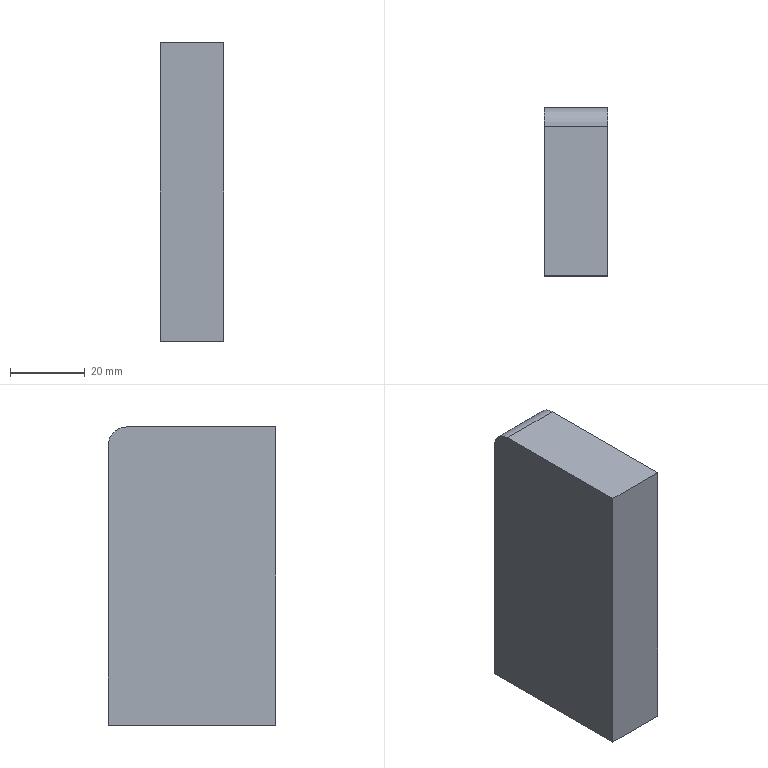Part | STEP file | DEWALT-DWE7492-B22 | 1 solid | 7 faces | box 17 x 45 x 80 mm | volume 61109 mm3 | plane 6 | cylinder 1 | commonest cylinder face diameters 10 x1
STEP:
#1=CARTESIAN_POINT('',(0.,0.,0.));
#2=DIRECTION('',(0.,0.,1.));
#3=DIRECTION('',(1.,0.,0.));
#4=AXIS2_PLACEMENT_3D('',#1,#2,#3);
#5=CARTESIAN_POINT('',(284.1,181.2,120.));
#6=VERTEX_POINT('',#5);
#7=CARTESIAN_POINT('',(284.1,186.2,115.));
#8=VERTEX_POINT('',#7);
#9=CARTESIAN_POINT('',(284.1,181.2,115.));
#10=DIRECTION('',(-1.,0.,0.));
#11=DIRECTION('',(0.,0.,1.));
#12=AXIS2_PLACEMENT_3D('',#9,#10,#11);
#13=CIRCLE('',#12,5.);
#14=CARTESIAN_POINT('',(284.1,181.2,115.));
#15=DIRECTION('',(-1.,0.,0.));
#16=DIRECTION('',(0.,0.,1.));
#17=AXIS2_PLACEMENT_3D('',#14,#15,#16);
#18=CYLINDRICAL_SURFACE('',#17,5.);
#19=CARTESIAN_POINT('',(0.,0.));
#20=DIRECTION('',(1.,0.));
#21=VECTOR('',#20,1.);
#22=LINE('',#19,#21);
#23=(GEOMETRIC_REPRESENTATION_CONTEXT(2)PARAMETRIC_REPRESENTATION_CONTEXT()REPRESENTATION_CONTEXT('',''));
#24=DEFINITIONAL_REPRESENTATION('',(#22),#23);
#25=PCURVE('',#18,#24);
#26=CARTESIAN_POINT('',(284.1,141.19,120.01));
#27=DIRECTION('',(1.,0.,0.));
#28=DIRECTION('',(0.,0.,-1.));
#29=AXIS2_PLACEMENT_3D('',#26,#27,#28);
#30=PLANE('',#29);
#31=CARTESIAN_POINT('',(0.01,40.01));
#32=CARTESIAN_POINT('',(0.01,48.67));
#33=CARTESIAN_POINT('',(7.51,44.34));
#34=CARTESIAN_POINT('',(15.01,40.01));
#35=CARTESIAN_POINT('',(7.51,35.68));
#36=CARTESIAN_POINT('',(0.01,31.35));
#37=CARTESIAN_POINT('',(0.01,40.01));
#38=(BOUNDED_CURVE()B_SPLINE_CURVE(2,(#31,#32,#33,#34,#35,#36,#37),.UNSPECIFIED.,.T.,.F.)B_SPLINE_CURVE_WITH_KNOTS((1,2,2,2,2,1),(-2.094,0.,2.094,4.189,6.283,8.378),.UNSPECIFIED.)CURVE()GEOMETRIC_REPRESENTATION_ITEM()RATIONAL_B_SPLINE_CURVE((1.,0.5,1.,0.5,1.,0.5,1.))REPRESENTATION_ITEM(''));
#39=(GEOMETRIC_REPRESENTATION_CONTEXT(2)PARAMETRIC_REPRESENTATION_CONTEXT()REPRESENTATION_CONTEXT('',''));
#40=DEFINITIONAL_REPRESENTATION('',(#38),#39);
#41=PCURVE('',#30,#40);
#42=SURFACE_CURVE('',#13,(#25,#41),.PCURVE_S1.);
#43=EDGE_CURVE('',#6,#8,#42,.T.);
#44=ORIENTED_EDGE('',*,*,#43,.T.);
#45=CARTESIAN_POINT('',(267.1,186.2,115.));
#46=VERTEX_POINT('',#45);
#47=CARTESIAN_POINT('',(275.6,186.2,115.));
#48=DIRECTION('',(-1.,0.,0.));
#49=VECTOR('',#48,1.);
#50=LINE('',#47,#49);
#51=CARTESIAN_POINT('',(1.571,8.5));
#52=DIRECTION('',(0.,1.));
#53=VECTOR('',#52,1.);
#54=LINE('',#51,#53);
#55=(GEOMETRIC_REPRESENTATION_CONTEXT(2)PARAMETRIC_REPRESENTATION_CONTEXT()REPRESENTATION_CONTEXT('',''));
#56=DEFINITIONAL_REPRESENTATION('',(#54),#55);
#57=PCURVE('',#18,#56);
#58=CARTESIAN_POINT('',(267.09,186.2,39.99));
#59=DIRECTION('',(0.,1.,0.));
#60=DIRECTION('',(0.,0.,1.));
#61=AXIS2_PLACEMENT_3D('',#58,#59,#60);
#62=PLANE('',#61);
#63=CARTESIAN_POINT('',(75.01,8.51));
#64=DIRECTION('',(0.,-1.));
#65=VECTOR('',#64,1.);
#66=LINE('',#63,#65);
#67=(GEOMETRIC_REPRESENTATION_CONTEXT(2)PARAMETRIC_REPRESENTATION_CONTEXT()REPRESENTATION_CONTEXT('',''));
#68=DEFINITIONAL_REPRESENTATION('',(#66),#67);
#69=PCURVE('',#62,#68);
#70=SURFACE_CURVE('',#50,(#57,#69),.PCURVE_S1.);
#71=EDGE_CURVE('',#8,#46,#70,.T.);
#72=ORIENTED_EDGE('',*,*,#71,.T.);
#73=CARTESIAN_POINT('',(267.1,181.2,120.));
#74=VERTEX_POINT('',#73);
#75=CARTESIAN_POINT('',(267.1,181.2,115.));
#76=DIRECTION('',(1.,0.,0.));
#77=DIRECTION('',(0.,1.,0.));
#78=AXIS2_PLACEMENT_3D('',#75,#76,#77);
#79=CIRCLE('',#78,5.);
#80=CARTESIAN_POINT('',(1.571,17.));
#81=DIRECTION('',(-1.,0.));
#82=VECTOR('',#81,1.);
#83=LINE('',#80,#82);
#84=(GEOMETRIC_REPRESENTATION_CONTEXT(2)PARAMETRIC_REPRESENTATION_CONTEXT()REPRESENTATION_CONTEXT('',''));
#85=DEFINITIONAL_REPRESENTATION('',(#83),#84);
#86=PCURVE('',#18,#85);
#87=CARTESIAN_POINT('',(267.1,186.21,39.99));
#88=DIRECTION('',(-1.,0.,0.));
#89=DIRECTION('',(0.,-1.,0.));
#90=AXIS2_PLACEMENT_3D('',#87,#88,#89);
#91=PLANE('',#90);
#92=CARTESIAN_POINT('',(0.01,75.01));
#93=CARTESIAN_POINT('',(0.01,83.67));
#94=CARTESIAN_POINT('',(7.51,79.34));
#95=CARTESIAN_POINT('',(15.01,75.01));
#96=CARTESIAN_POINT('',(7.51,70.68));
#97=CARTESIAN_POINT('',(0.01,66.35));
#98=CARTESIAN_POINT('',(0.01,75.01));
#99=(BOUNDED_CURVE()B_SPLINE_CURVE(2,(#92,#93,#94,#95,#96,#97,#98),.UNSPECIFIED.,.T.,.F.)B_SPLINE_CURVE_WITH_KNOTS((1,2,2,2,2,1),(-2.094,0.,2.094,4.189,6.283,8.378),.UNSPECIFIED.)CURVE()GEOMETRIC_REPRESENTATION_ITEM()RATIONAL_B_SPLINE_CURVE((1.,0.5,1.,0.5,1.,0.5,1.))REPRESENTATION_ITEM(''));
#100=(GEOMETRIC_REPRESENTATION_CONTEXT(2)PARAMETRIC_REPRESENTATION_CONTEXT()REPRESENTATION_CONTEXT('',''));
#101=DEFINITIONAL_REPRESENTATION('',(#99),#100);
#102=PCURVE('',#91,#101);
#103=SURFACE_CURVE('',#79,(#86,#102),.PCURVE_S1.);
#104=EDGE_CURVE('',#46,#74,#103,.T.);
#105=ORIENTED_EDGE('',*,*,#104,.T.);
#106=CARTESIAN_POINT('',(275.6,181.2,120.));
#107=DIRECTION('',(1.,0.,0.));
#108=VECTOR('',#107,1.);
#109=LINE('',#106,#108);
#110=CARTESIAN_POINT('',(0.,8.5));
#111=DIRECTION('',(0.,-1.));
#112=VECTOR('',#111,1.);
#113=LINE('',#110,#112);
#114=(GEOMETRIC_REPRESENTATION_CONTEXT(2)PARAMETRIC_REPRESENTATION_CONTEXT()REPRESENTATION_CONTEXT('',''));
#115=DEFINITIONAL_REPRESENTATION('',(#113),#114);
#116=PCURVE('',#18,#115);
#117=CARTESIAN_POINT('',(267.09,181.21,120.));
#118=DIRECTION('',(0.,0.,1.));
#119=DIRECTION('',(0.,-1.,0.));
#120=AXIS2_PLACEMENT_3D('',#117,#118,#119);
#121=PLANE('',#120);
#122=CARTESIAN_POINT('',(0.01,8.51));
#123=DIRECTION('',(0.,1.));
#124=VECTOR('',#123,1.);
#125=LINE('',#122,#124);
#126=(GEOMETRIC_REPRESENTATION_CONTEXT(2)PARAMETRIC_REPRESENTATION_CONTEXT()REPRESENTATION_CONTEXT('',''));
#127=DEFINITIONAL_REPRESENTATION('',(#125),#126);
#128=PCURVE('',#121,#127);
#129=SURFACE_CURVE('',#109,(#116,#128),.PCURVE_S1.);
#130=EDGE_CURVE('',#74,#6,#129,.T.);
#131=ORIENTED_EDGE('',*,*,#130,.T.);
#132=EDGE_LOOP('',(#44,#72,#105,#131));
#133=FACE_BOUND('',#132,.T.);
#134=ADVANCED_FACE('',(#133),#18,.T.);
#135=ORIENTED_EDGE('',*,*,#104,.F.);
#136=CARTESIAN_POINT('',(267.1,186.2,40.));
#137=VERTEX_POINT('',#136);
#138=CARTESIAN_POINT('',(267.1,186.2,77.5));
#139=DIRECTION('',(0.,0.,1.));
#140=VECTOR('',#139,1.);
#141=LINE('',#138,#140);
#142=CARTESIAN_POINT('',(0.01,37.51));
#143=DIRECTION('',(0.,1.));
#144=VECTOR('',#143,1.);
#145=LINE('',#142,#144);
#146=(GEOMETRIC_REPRESENTATION_CONTEXT(2)PARAMETRIC_REPRESENTATION_CONTEXT()REPRESENTATION_CONTEXT('',''));
#147=DEFINITIONAL_REPRESENTATION('',(#145),#146);
#148=PCURVE('',#91,#147);
#149=CARTESIAN_POINT('',(37.51,0.01));
#150=DIRECTION('',(1.,0.));
#151=VECTOR('',#150,1.);
#152=LINE('',#149,#151);
#153=(GEOMETRIC_REPRESENTATION_CONTEXT(2)PARAMETRIC_REPRESENTATION_CONTEXT()REPRESENTATION_CONTEXT('',''));
#154=DEFINITIONAL_REPRESENTATION('',(#152),#153);
#155=PCURVE('',#62,#154);
#156=SURFACE_CURVE('',#141,(#148,#155),.PCURVE_S1.);
#157=EDGE_CURVE('',#137,#46,#156,.T.);
#158=ORIENTED_EDGE('',*,*,#157,.F.);
#159=CARTESIAN_POINT('',(267.1,141.2,40.));
#160=VERTEX_POINT('',#159);
#161=CARTESIAN_POINT('',(267.1,163.7,40.));
#162=DIRECTION('',(0.,1.,0.));
#163=VECTOR('',#162,1.);
#164=LINE('',#161,#163);
#165=CARTESIAN_POINT('',(22.51,0.01));
#166=DIRECTION('',(-1.,0.));
#167=VECTOR('',#166,1.);
#168=LINE('',#165,#167);
#169=(GEOMETRIC_REPRESENTATION_CONTEXT(2)PARAMETRIC_REPRESENTATION_CONTEXT()REPRESENTATION_CONTEXT('',''));
#170=DEFINITIONAL_REPRESENTATION('',(#168),#169);
#171=PCURVE('',#91,#170);
#172=CARTESIAN_POINT('',(267.09,141.19,40.));
#173=DIRECTION('',(0.,0.,-1.));
#174=DIRECTION('',(0.,1.,0.));
#175=AXIS2_PLACEMENT_3D('',#172,#173,#174);
#176=PLANE('',#175);
#177=CARTESIAN_POINT('',(22.51,0.01));
#178=DIRECTION('',(1.,0.));
#179=VECTOR('',#178,1.);
#180=LINE('',#177,#179);
#181=(GEOMETRIC_REPRESENTATION_CONTEXT(2)PARAMETRIC_REPRESENTATION_CONTEXT()REPRESENTATION_CONTEXT('',''));
#182=DEFINITIONAL_REPRESENTATION('',(#180),#181);
#183=PCURVE('',#176,#182);
#184=SURFACE_CURVE('',#164,(#171,#183),.PCURVE_S1.);
#185=EDGE_CURVE('',#160,#137,#184,.T.);
#186=ORIENTED_EDGE('',*,*,#185,.F.);
#187=CARTESIAN_POINT('',(267.1,141.2,120.));
#188=VERTEX_POINT('',#187);
#189=CARTESIAN_POINT('',(267.1,141.2,80.));
#190=DIRECTION('',(0.,0.,-1.));
#191=VECTOR('',#190,1.);
#192=LINE('',#189,#191);
#193=CARTESIAN_POINT('',(45.01,40.01));
#194=DIRECTION('',(0.,-1.));
#195=VECTOR('',#194,1.);
#196=LINE('',#193,#195);
#197=(GEOMETRIC_REPRESENTATION_CONTEXT(2)PARAMETRIC_REPRESENTATION_CONTEXT()REPRESENTATION_CONTEXT('',''));
#198=DEFINITIONAL_REPRESENTATION('',(#196),#197);
#199=PCURVE('',#91,#198);
#200=CARTESIAN_POINT('',(267.09,141.2,120.01));
#201=DIRECTION('',(0.,-1.,0.));
#202=DIRECTION('',(0.,0.,-1.));
#203=AXIS2_PLACEMENT_3D('',#200,#201,#202);
#204=PLANE('',#203);
#205=CARTESIAN_POINT('',(40.01,0.01));
#206=DIRECTION('',(1.,0.));
#207=VECTOR('',#206,1.);
#208=LINE('',#205,#207);
#209=(GEOMETRIC_REPRESENTATION_CONTEXT(2)PARAMETRIC_REPRESENTATION_CONTEXT()REPRESENTATION_CONTEXT('',''));
#210=DEFINITIONAL_REPRESENTATION('',(#208),#209);
#211=PCURVE('',#204,#210);
#212=SURFACE_CURVE('',#192,(#199,#211),.PCURVE_S1.);
#213=EDGE_CURVE('',#188,#160,#212,.T.);
#214=ORIENTED_EDGE('',*,*,#213,.F.);
#215=CARTESIAN_POINT('',(267.1,161.2,120.));
#216=DIRECTION('',(0.,-1.,0.));
#217=VECTOR('',#216,1.);
#218=LINE('',#215,#217);
#219=CARTESIAN_POINT('',(25.01,80.01));
#220=DIRECTION('',(1.,0.));
#221=VECTOR('',#220,1.);
#222=LINE('',#219,#221);
#223=(GEOMETRIC_REPRESENTATION_CONTEXT(2)PARAMETRIC_REPRESENTATION_CONTEXT()REPRESENTATION_CONTEXT('',''));
#224=DEFINITIONAL_REPRESENTATION('',(#222),#223);
#225=PCURVE('',#91,#224);
#226=CARTESIAN_POINT('',(20.01,0.01));
#227=DIRECTION('',(1.,0.));
#228=VECTOR('',#227,1.);
#229=LINE('',#226,#228);
#230=(GEOMETRIC_REPRESENTATION_CONTEXT(2)PARAMETRIC_REPRESENTATION_CONTEXT()REPRESENTATION_CONTEXT('',''));
#231=DEFINITIONAL_REPRESENTATION('',(#229),#230);
#232=PCURVE('',#121,#231);
#233=SURFACE_CURVE('',#218,(#225,#232),.PCURVE_S1.);
#234=EDGE_CURVE('',#74,#188,#233,.T.);
#235=ORIENTED_EDGE('',*,*,#234,.F.);
#236=EDGE_LOOP('',(#135,#158,#186,#214,#235));
#237=FACE_BOUND('',#236,.T.);
#238=ADVANCED_FACE('',(#237),#91,.T.);
#239=ORIENTED_EDGE('',*,*,#71,.F.);
#240=CARTESIAN_POINT('',(284.1,186.2,40.));
#241=VERTEX_POINT('',#240);
#242=CARTESIAN_POINT('',(284.1,186.2,77.5));
#243=DIRECTION('',(0.,0.,1.));
#244=VECTOR('',#243,1.);
#245=LINE('',#242,#244);
#246=CARTESIAN_POINT('',(37.51,17.01));
#247=DIRECTION('',(1.,0.));
#248=VECTOR('',#247,1.);
#249=LINE('',#246,#248);
#250=(GEOMETRIC_REPRESENTATION_CONTEXT(2)PARAMETRIC_REPRESENTATION_CONTEXT()REPRESENTATION_CONTEXT('',''));
#251=DEFINITIONAL_REPRESENTATION('',(#249),#250);
#252=PCURVE('',#62,#251);
#253=CARTESIAN_POINT('',(42.51,45.01));
#254=DIRECTION('',(-1.,0.));
#255=VECTOR('',#254,1.);
#256=LINE('',#253,#255);
#257=(GEOMETRIC_REPRESENTATION_CONTEXT(2)PARAMETRIC_REPRESENTATION_CONTEXT()REPRESENTATION_CONTEXT('',''));
#258=DEFINITIONAL_REPRESENTATION('',(#256),#257);
#259=PCURVE('',#30,#258);
#260=SURFACE_CURVE('',#245,(#252,#259),.PCURVE_S1.);
#261=EDGE_CURVE('',#241,#8,#260,.T.);
#262=ORIENTED_EDGE('',*,*,#261,.F.);
#263=CARTESIAN_POINT('',(275.6,186.2,40.));
#264=DIRECTION('',(1.,0.,0.));
#265=VECTOR('',#264,1.);
#266=LINE('',#263,#265);
#267=CARTESIAN_POINT('',(0.01,8.51));
#268=DIRECTION('',(0.,1.));
#269=VECTOR('',#268,1.);
#270=LINE('',#267,#269);
#271=(GEOMETRIC_REPRESENTATION_CONTEXT(2)PARAMETRIC_REPRESENTATION_CONTEXT()REPRESENTATION_CONTEXT('',''));
#272=DEFINITIONAL_REPRESENTATION('',(#270),#271);
#273=PCURVE('',#62,#272);
#274=CARTESIAN_POINT('',(45.01,8.51));
#275=DIRECTION('',(0.,1.));
#276=VECTOR('',#275,1.);
#277=LINE('',#274,#276);
#278=(GEOMETRIC_REPRESENTATION_CONTEXT(2)PARAMETRIC_REPRESENTATION_CONTEXT()REPRESENTATION_CONTEXT('',''));
#279=DEFINITIONAL_REPRESENTATION('',(#277),#278);
#280=PCURVE('',#176,#279);
#281=SURFACE_CURVE('',#266,(#273,#280),.PCURVE_S1.);
#282=EDGE_CURVE('',#137,#241,#281,.T.);
#283=ORIENTED_EDGE('',*,*,#282,.F.);
#284=ORIENTED_EDGE('',*,*,#157,.T.);
#285=EDGE_LOOP('',(#239,#262,#283,#284));
#286=FACE_BOUND('',#285,.T.);
#287=ADVANCED_FACE('',(#286),#62,.T.);
#288=ORIENTED_EDGE('',*,*,#130,.F.);
#289=ORIENTED_EDGE('',*,*,#234,.T.);
#290=CARTESIAN_POINT('',(284.1,141.2,120.));
#291=VERTEX_POINT('',#290);
#292=CARTESIAN_POINT('',(275.6,141.2,120.));
#293=DIRECTION('',(1.,0.,0.));
#294=VECTOR('',#293,1.);
#295=LINE('',#292,#294);
#296=CARTESIAN_POINT('',(40.01,8.51));
#297=DIRECTION('',(0.,1.));
#298=VECTOR('',#297,1.);
#299=LINE('',#296,#298);
#300=(GEOMETRIC_REPRESENTATION_CONTEXT(2)PARAMETRIC_REPRESENTATION_CONTEXT()REPRESENTATION_CONTEXT('',''));
#301=DEFINITIONAL_REPRESENTATION('',(#299),#300);
#302=PCURVE('',#121,#301);
#303=CARTESIAN_POINT('',(0.01,8.51));
#304=DIRECTION('',(0.,1.));
#305=VECTOR('',#304,1.);
#306=LINE('',#303,#305);
#307=(GEOMETRIC_REPRESENTATION_CONTEXT(2)PARAMETRIC_REPRESENTATION_CONTEXT()REPRESENTATION_CONTEXT('',''));
#308=DEFINITIONAL_REPRESENTATION('',(#306),#307);
#309=PCURVE('',#204,#308);
#310=SURFACE_CURVE('',#295,(#302,#309),.PCURVE_S1.);
#311=EDGE_CURVE('',#188,#291,#310,.T.);
#312=ORIENTED_EDGE('',*,*,#311,.T.);
#313=CARTESIAN_POINT('',(284.1,161.2,120.));
#314=DIRECTION('',(0.,-1.,0.));
#315=VECTOR('',#314,1.);
#316=LINE('',#313,#315);
#317=CARTESIAN_POINT('',(20.01,17.01));
#318=DIRECTION('',(1.,0.));
#319=VECTOR('',#318,1.);
#320=LINE('',#317,#319);
#321=(GEOMETRIC_REPRESENTATION_CONTEXT(2)PARAMETRIC_REPRESENTATION_CONTEXT()REPRESENTATION_CONTEXT('',''));
#322=DEFINITIONAL_REPRESENTATION('',(#320),#321);
#323=PCURVE('',#121,#322);
#324=CARTESIAN_POINT('',(0.01,20.01));
#325=DIRECTION('',(0.,-1.));
#326=VECTOR('',#325,1.);
#327=LINE('',#324,#326);
#328=(GEOMETRIC_REPRESENTATION_CONTEXT(2)PARAMETRIC_REPRESENTATION_CONTEXT()REPRESENTATION_CONTEXT('',''));
#329=DEFINITIONAL_REPRESENTATION('',(#327),#328);
#330=PCURVE('',#30,#329);
#331=SURFACE_CURVE('',#316,(#323,#330),.PCURVE_S1.);
#332=EDGE_CURVE('',#6,#291,#331,.T.);
#333=ORIENTED_EDGE('',*,*,#332,.F.);
#334=EDGE_LOOP('',(#288,#289,#312,#333));
#335=FACE_BOUND('',#334,.T.);
#336=ADVANCED_FACE('',(#335),#121,.T.);
#337=ORIENTED_EDGE('',*,*,#185,.T.);
#338=ORIENTED_EDGE('',*,*,#282,.T.);
#339=CARTESIAN_POINT('',(284.1,141.2,40.));
#340=VERTEX_POINT('',#339);
#341=CARTESIAN_POINT('',(284.1,163.7,40.));
#342=DIRECTION('',(0.,1.,0.));
#343=VECTOR('',#342,1.);
#344=LINE('',#341,#343);
#345=CARTESIAN_POINT('',(22.51,17.01));
#346=DIRECTION('',(1.,0.));
#347=VECTOR('',#346,1.);
#348=LINE('',#345,#347);
#349=(GEOMETRIC_REPRESENTATION_CONTEXT(2)PARAMETRIC_REPRESENTATION_CONTEXT()REPRESENTATION_CONTEXT('',''));
#350=DEFINITIONAL_REPRESENTATION('',(#348),#349);
#351=PCURVE('',#176,#350);
#352=CARTESIAN_POINT('',(80.01,22.51));
#353=DIRECTION('',(0.,1.));
#354=VECTOR('',#353,1.);
#355=LINE('',#352,#354);
#356=(GEOMETRIC_REPRESENTATION_CONTEXT(2)PARAMETRIC_REPRESENTATION_CONTEXT()REPRESENTATION_CONTEXT('',''));
#357=DEFINITIONAL_REPRESENTATION('',(#355),#356);
#358=PCURVE('',#30,#357);
#359=SURFACE_CURVE('',#344,(#351,#358),.PCURVE_S1.);
#360=EDGE_CURVE('',#340,#241,#359,.T.);
#361=ORIENTED_EDGE('',*,*,#360,.F.);
#362=CARTESIAN_POINT('',(275.6,141.2,40.));
#363=DIRECTION('',(1.,0.,0.));
#364=VECTOR('',#363,1.);
#365=LINE('',#362,#364);
#366=CARTESIAN_POINT('',(0.01,8.51));
#367=DIRECTION('',(0.,1.));
#368=VECTOR('',#367,1.);
#369=LINE('',#366,#368);
#370=(GEOMETRIC_REPRESENTATION_CONTEXT(2)PARAMETRIC_REPRESENTATION_CONTEXT()REPRESENTATION_CONTEXT('',''));
#371=DEFINITIONAL_REPRESENTATION('',(#369),#370);
#372=PCURVE('',#176,#371);
#373=CARTESIAN_POINT('',(80.01,8.51));
#374=DIRECTION('',(0.,1.));
#375=VECTOR('',#374,1.);
#376=LINE('',#373,#375);
#377=(GEOMETRIC_REPRESENTATION_CONTEXT(2)PARAMETRIC_REPRESENTATION_CONTEXT()REPRESENTATION_CONTEXT('',''));
#378=DEFINITIONAL_REPRESENTATION('',(#376),#377);
#379=PCURVE('',#204,#378);
#380=SURFACE_CURVE('',#365,(#372,#379),.PCURVE_S1.);
#381=EDGE_CURVE('',#160,#340,#380,.T.);
#382=ORIENTED_EDGE('',*,*,#381,.F.);
#383=EDGE_LOOP('',(#337,#338,#361,#382));
#384=FACE_BOUND('',#383,.T.);
#385=ADVANCED_FACE('',(#384),#176,.T.);
#386=ORIENTED_EDGE('',*,*,#213,.T.);
#387=ORIENTED_EDGE('',*,*,#381,.T.);
#388=CARTESIAN_POINT('',(284.1,141.2,80.));
#389=DIRECTION('',(0.,0.,-1.));
#390=VECTOR('',#389,1.);
#391=LINE('',#388,#390);
#392=CARTESIAN_POINT('',(40.01,17.01));
#393=DIRECTION('',(1.,0.));
#394=VECTOR('',#393,1.);
#395=LINE('',#392,#394);
#396=(GEOMETRIC_REPRESENTATION_CONTEXT(2)PARAMETRIC_REPRESENTATION_CONTEXT()REPRESENTATION_CONTEXT('',''));
#397=DEFINITIONAL_REPRESENTATION('',(#395),#396);
#398=PCURVE('',#204,#397);
#399=CARTESIAN_POINT('',(40.01,0.01));
#400=DIRECTION('',(1.,0.));
#401=VECTOR('',#400,1.);
#402=LINE('',#399,#401);
#403=(GEOMETRIC_REPRESENTATION_CONTEXT(2)PARAMETRIC_REPRESENTATION_CONTEXT()REPRESENTATION_CONTEXT('',''));
#404=DEFINITIONAL_REPRESENTATION('',(#402),#403);
#405=PCURVE('',#30,#404);
#406=SURFACE_CURVE('',#391,(#398,#405),.PCURVE_S1.);
#407=EDGE_CURVE('',#291,#340,#406,.T.);
#408=ORIENTED_EDGE('',*,*,#407,.F.);
#409=ORIENTED_EDGE('',*,*,#311,.F.);
#410=EDGE_LOOP('',(#386,#387,#408,#409));
#411=FACE_BOUND('',#410,.T.);
#412=ADVANCED_FACE('',(#411),#204,.T.);
#413=ORIENTED_EDGE('',*,*,#43,.F.);
#414=ORIENTED_EDGE('',*,*,#332,.T.);
#415=ORIENTED_EDGE('',*,*,#407,.T.);
#416=ORIENTED_EDGE('',*,*,#360,.T.);
#417=ORIENTED_EDGE('',*,*,#261,.T.);
#418=EDGE_LOOP('',(#413,#414,#415,#416,#417));
#419=FACE_BOUND('',#418,.T.);
#420=ADVANCED_FACE('',(#419),#30,.T.);
#421=CLOSED_SHELL('',(#134,#238,#287,#336,#385,#412,#420));
#422=MANIFOLD_SOLID_BREP('',#421);
#423=(LENGTH_UNIT()NAMED_UNIT(*)SI_UNIT(.MILLI.,.METRE.));
#424=UNCERTAINTY_MEASURE_WITH_UNIT(LENGTH_MEASURE(0.0000001),#423,'','');
#425=(NAMED_UNIT(*)PLANE_ANGLE_UNIT()SI_UNIT($,.RADIAN.));
#426=(NAMED_UNIT(*)SI_UNIT($,.STERADIAN.)SOLID_ANGLE_UNIT());
#427=(GEOMETRIC_REPRESENTATION_CONTEXT(3)GLOBAL_UNCERTAINTY_ASSIGNED_CONTEXT((#424))GLOBAL_UNIT_ASSIGNED_CONTEXT((#423,#425,#426))REPRESENTATION_CONTEXT('',''));
#428=ADVANCED_BREP_SHAPE_REPRESENTATION('',(#4,#422),#427);